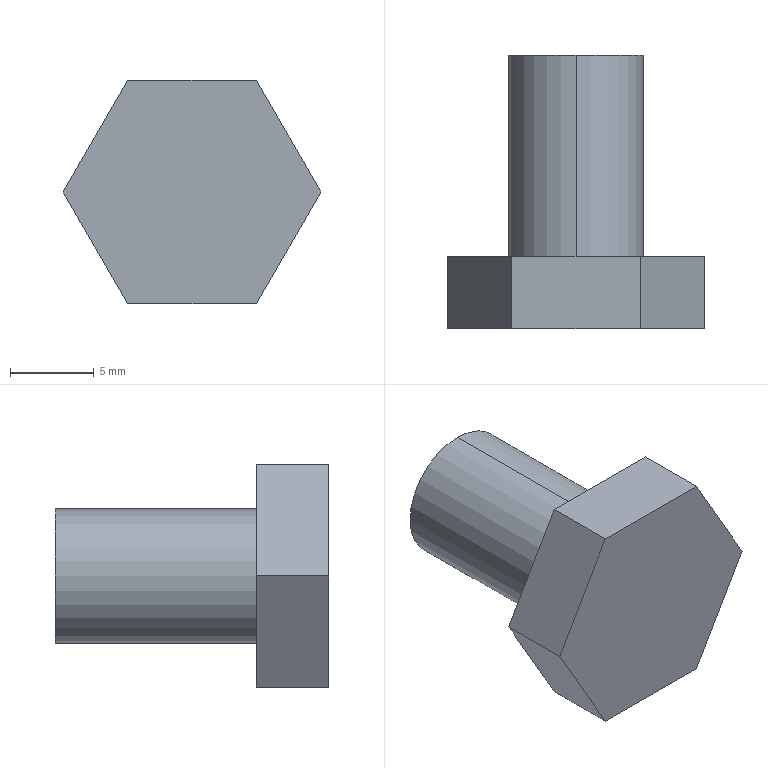Part | SolidWorks | features BaseBody 1 | 1 solid | 11 faces | box 15.358 x 16.3 x 13.3 mm | volume 1262 mm3 | plane 9 | cylinder 2 | commonest cylinder face diameters 8 x2
STEP:
#1=CARTESIAN_POINT('',(0.,16.3,-4.));
#2=VERTEX_POINT('',#1);
#3=CARTESIAN_POINT('',(0.,16.3,4.));
#4=VERTEX_POINT('',#3);
#5=CARTESIAN_POINT('',(0.,16.3,0.));
#6=DIRECTION('',(0.,-1.,0.));
#7=DIRECTION('',(0.,0.,-1.));
#8=AXIS2_PLACEMENT_3D('',#5,#6,#7);
#9=CIRCLE('',#8,4.);
#10=EDGE_CURVE('',#2,#4,#9,.T.);
#11=ORIENTED_EDGE('',*,*,#10,.T.);
#12=CARTESIAN_POINT('',(0.,4.3,4.));
#13=VERTEX_POINT('',#12);
#14=CARTESIAN_POINT('',(0.,16.3,4.));
#15=DIRECTION('',(0.,-1.,0.));
#16=VECTOR('',#15,1000.);
#17=LINE('',#14,#16);
#18=EDGE_CURVE('',#4,#13,#17,.T.);
#19=ORIENTED_EDGE('',*,*,#18,.T.);
#20=CARTESIAN_POINT('',(0.,4.3,-4.));
#21=VERTEX_POINT('',#20);
#22=CARTESIAN_POINT('',(0.,4.3,0.));
#23=DIRECTION('',(0.,-1.,0.));
#24=DIRECTION('',(0.,0.,-1.));
#25=AXIS2_PLACEMENT_3D('',#22,#23,#24);
#26=CIRCLE('',#25,4.);
#27=EDGE_CURVE('',#21,#13,#26,.T.);
#28=ORIENTED_EDGE('',*,*,#27,.F.);
#29=CARTESIAN_POINT('',(0.,16.3,-4.));
#30=DIRECTION('',(0.,-1.,0.));
#31=VECTOR('',#30,1000.);
#32=LINE('',#29,#31);
#33=EDGE_CURVE('',#2,#21,#32,.T.);
#34=ORIENTED_EDGE('',*,*,#33,.F.);
#35=EDGE_LOOP('',(#11,#19,#28,#34));
#36=FACE_OUTER_BOUND('',#35,.T.);
#37=CARTESIAN_POINT('',(0.,16.3,0.));
#38=DIRECTION('',(0.,-1.,0.));
#39=DIRECTION('',(0.,0.,-1.));
#40=AXIS2_PLACEMENT_3D('',#37,#38,#39);
#41=CYLINDRICAL_SURFACE('',#40,4.);
#42=ADVANCED_FACE('',(#36),#41,.T.);
#43=CARTESIAN_POINT('',(-3.839,0.,6.65));
#44=VERTEX_POINT('',#43);
#45=CARTESIAN_POINT('',(3.839,0.,6.65));
#46=VERTEX_POINT('',#45);
#47=CARTESIAN_POINT('',(0.,0.,6.65));
#48=DIRECTION('',(1.,0.,0.));
#49=VECTOR('',#48,1000.);
#50=LINE('',#47,#49);
#51=EDGE_CURVE('',#44,#46,#50,.T.);
#52=ORIENTED_EDGE('',*,*,#51,.F.);
#53=CARTESIAN_POINT('',(-7.679,0.,0.));
#54=VERTEX_POINT('',#53);
#55=CARTESIAN_POINT('',(-7.679,0.,0.));
#56=DIRECTION('',(0.5,0.,0.866));
#57=VECTOR('',#56,1000.);
#58=LINE('',#55,#57);
#59=EDGE_CURVE('',#54,#44,#58,.T.);
#60=ORIENTED_EDGE('',*,*,#59,.F.);
#61=CARTESIAN_POINT('',(-3.839,0.,-6.65));
#62=VERTEX_POINT('',#61);
#63=CARTESIAN_POINT('',(-3.839,0.,-6.65));
#64=DIRECTION('',(-0.5,0.,0.866));
#65=VECTOR('',#64,1000.);
#66=LINE('',#63,#65);
#67=EDGE_CURVE('',#62,#54,#66,.T.);
#68=ORIENTED_EDGE('',*,*,#67,.F.);
#69=CARTESIAN_POINT('',(3.839,0.,-6.65));
#70=VERTEX_POINT('',#69);
#71=CARTESIAN_POINT('',(0.,0.,-6.65));
#72=DIRECTION('',(-1.,0.,0.));
#73=VECTOR('',#72,1000.);
#74=LINE('',#71,#73);
#75=EDGE_CURVE('',#70,#62,#74,.T.);
#76=ORIENTED_EDGE('',*,*,#75,.F.);
#77=CARTESIAN_POINT('',(7.679,0.,0.));
#78=VERTEX_POINT('',#77);
#79=CARTESIAN_POINT('',(7.679,0.,0.));
#80=DIRECTION('',(-0.5,0.,-0.866));
#81=VECTOR('',#80,1000.);
#82=LINE('',#79,#81);
#83=EDGE_CURVE('',#78,#70,#82,.T.);
#84=ORIENTED_EDGE('',*,*,#83,.F.);
#85=CARTESIAN_POINT('',(3.839,0.,6.65));
#86=DIRECTION('',(0.5,0.,-0.866));
#87=VECTOR('',#86,1000.);
#88=LINE('',#85,#87);
#89=EDGE_CURVE('',#46,#78,#88,.T.);
#90=ORIENTED_EDGE('',*,*,#89,.F.);
#91=EDGE_LOOP('',(#52,#60,#68,#76,#84,#90));
#92=FACE_OUTER_BOUND('',#91,.T.);
#93=CARTESIAN_POINT('',(0.,0.,0.));
#94=DIRECTION('',(0.,1.,0.));
#95=DIRECTION('',(0.,0.,1.));
#96=AXIS2_PLACEMENT_3D('',#93,#94,#95);
#97=PLANE('',#96);
#98=ADVANCED_FACE('',(#92),#97,.F.);
#99=CARTESIAN_POINT('',(7.679,4.3,0.));
#100=VERTEX_POINT('',#99);
#101=CARTESIAN_POINT('',(7.679,4.3,0.));
#102=DIRECTION('',(0.,-1.,0.));
#103=VECTOR('',#102,1000.);
#104=LINE('',#101,#103);
#105=EDGE_CURVE('',#100,#78,#104,.T.);
#106=ORIENTED_EDGE('',*,*,#105,.F.);
#107=CARTESIAN_POINT('',(3.839,4.3,6.65));
#108=VERTEX_POINT('',#107);
#109=CARTESIAN_POINT('',(3.839,4.3,6.65));
#110=DIRECTION('',(0.5,0.,-0.866));
#111=VECTOR('',#110,1000.);
#112=LINE('',#109,#111);
#113=EDGE_CURVE('',#108,#100,#112,.T.);
#114=ORIENTED_EDGE('',*,*,#113,.F.);
#115=CARTESIAN_POINT('',(3.839,4.3,6.65));
#116=DIRECTION('',(0.,1.,0.));
#117=VECTOR('',#116,1000.);
#118=LINE('',#115,#117);
#119=EDGE_CURVE('',#46,#108,#118,.T.);
#120=ORIENTED_EDGE('',*,*,#119,.F.);
#121=ORIENTED_EDGE('',*,*,#89,.T.);
#122=EDGE_LOOP('',(#106,#114,#120,#121));
#123=FACE_OUTER_BOUND('',#122,.T.);
#124=CARTESIAN_POINT('',(3.839,4.3,6.65));
#125=DIRECTION('',(-0.866,0.,-0.5));
#126=DIRECTION('',(-0.5,0.,0.866));
#127=AXIS2_PLACEMENT_3D('',#124,#125,#126);
#128=PLANE('',#127);
#129=ADVANCED_FACE('',(#123),#128,.F.);
#130=ORIENTED_EDGE('',*,*,#119,.T.);
#131=CARTESIAN_POINT('',(-3.839,4.3,6.65));
#132=VERTEX_POINT('',#131);
#133=CARTESIAN_POINT('',(-3.839,4.3,6.65));
#134=DIRECTION('',(1.,0.,0.));
#135=VECTOR('',#134,1000.);
#136=LINE('',#133,#135);
#137=EDGE_CURVE('',#132,#108,#136,.T.);
#138=ORIENTED_EDGE('',*,*,#137,.F.);
#139=CARTESIAN_POINT('',(-3.839,4.3,6.65));
#140=DIRECTION('',(0.,1.,0.));
#141=VECTOR('',#140,1000.);
#142=LINE('',#139,#141);
#143=EDGE_CURVE('',#44,#132,#142,.T.);
#144=ORIENTED_EDGE('',*,*,#143,.F.);
#145=ORIENTED_EDGE('',*,*,#51,.T.);
#146=EDGE_LOOP('',(#130,#138,#144,#145));
#147=FACE_OUTER_BOUND('',#146,.T.);
#148=CARTESIAN_POINT('',(-3.839,4.3,6.65));
#149=DIRECTION('',(0.,0.,-1.));
#150=DIRECTION('',(-1.,0.,0.));
#151=AXIS2_PLACEMENT_3D('',#148,#149,#150);
#152=PLANE('',#151);
#153=ADVANCED_FACE('',(#147),#152,.F.);
#154=ORIENTED_EDGE('',*,*,#143,.T.);
#155=CARTESIAN_POINT('',(-7.679,4.3,0.));
#156=VERTEX_POINT('',#155);
#157=CARTESIAN_POINT('',(-7.679,4.3,0.));
#158=DIRECTION('',(0.5,0.,0.866));
#159=VECTOR('',#158,1000.);
#160=LINE('',#157,#159);
#161=EDGE_CURVE('',#156,#132,#160,.T.);
#162=ORIENTED_EDGE('',*,*,#161,.F.);
#163=CARTESIAN_POINT('',(-7.679,4.3,0.));
#164=DIRECTION('',(0.,1.,0.));
#165=VECTOR('',#164,1000.);
#166=LINE('',#163,#165);
#167=EDGE_CURVE('',#54,#156,#166,.T.);
#168=ORIENTED_EDGE('',*,*,#167,.F.);
#169=ORIENTED_EDGE('',*,*,#59,.T.);
#170=EDGE_LOOP('',(#154,#162,#168,#169));
#171=FACE_OUTER_BOUND('',#170,.T.);
#172=CARTESIAN_POINT('',(-7.679,4.3,0.));
#173=DIRECTION('',(0.866,0.,-0.5));
#174=DIRECTION('',(-0.5,0.,-0.866));
#175=AXIS2_PLACEMENT_3D('',#172,#173,#174);
#176=PLANE('',#175);
#177=ADVANCED_FACE('',(#171),#176,.F.);
#178=ORIENTED_EDGE('',*,*,#167,.T.);
#179=CARTESIAN_POINT('',(-3.839,4.3,-6.65));
#180=VERTEX_POINT('',#179);
#181=CARTESIAN_POINT('',(-3.839,4.3,-6.65));
#182=DIRECTION('',(-0.5,0.,0.866));
#183=VECTOR('',#182,1000.);
#184=LINE('',#181,#183);
#185=EDGE_CURVE('',#180,#156,#184,.T.);
#186=ORIENTED_EDGE('',*,*,#185,.F.);
#187=CARTESIAN_POINT('',(-3.839,4.3,-6.65));
#188=DIRECTION('',(0.,1.,0.));
#189=VECTOR('',#188,1000.);
#190=LINE('',#187,#189);
#191=EDGE_CURVE('',#62,#180,#190,.T.);
#192=ORIENTED_EDGE('',*,*,#191,.F.);
#193=ORIENTED_EDGE('',*,*,#67,.T.);
#194=EDGE_LOOP('',(#178,#186,#192,#193));
#195=FACE_OUTER_BOUND('',#194,.T.);
#196=CARTESIAN_POINT('',(-3.839,4.3,-6.65));
#197=DIRECTION('',(0.866,0.,0.5));
#198=DIRECTION('',(0.5,0.,-0.866));
#199=AXIS2_PLACEMENT_3D('',#196,#197,#198);
#200=PLANE('',#199);
#201=ADVANCED_FACE('',(#195),#200,.F.);
#202=ORIENTED_EDGE('',*,*,#191,.T.);
#203=CARTESIAN_POINT('',(3.839,4.3,-6.65));
#204=VERTEX_POINT('',#203);
#205=CARTESIAN_POINT('',(3.839,4.3,-6.65));
#206=DIRECTION('',(-1.,0.,0.));
#207=VECTOR('',#206,1000.);
#208=LINE('',#205,#207);
#209=EDGE_CURVE('',#204,#180,#208,.T.);
#210=ORIENTED_EDGE('',*,*,#209,.F.);
#211=CARTESIAN_POINT('',(3.839,4.3,-6.65));
#212=DIRECTION('',(0.,1.,0.));
#213=VECTOR('',#212,1000.);
#214=LINE('',#211,#213);
#215=EDGE_CURVE('',#70,#204,#214,.T.);
#216=ORIENTED_EDGE('',*,*,#215,.F.);
#217=ORIENTED_EDGE('',*,*,#75,.T.);
#218=EDGE_LOOP('',(#202,#210,#216,#217));
#219=FACE_OUTER_BOUND('',#218,.T.);
#220=CARTESIAN_POINT('',(3.839,4.3,-6.65));
#221=DIRECTION('',(0.,0.,1.));
#222=DIRECTION('',(1.,0.,0.));
#223=AXIS2_PLACEMENT_3D('',#220,#221,#222);
#224=PLANE('',#223);
#225=ADVANCED_FACE('',(#219),#224,.F.);
#226=ORIENTED_EDGE('',*,*,#215,.T.);
#227=CARTESIAN_POINT('',(7.679,4.3,0.));
#228=DIRECTION('',(-0.5,0.,-0.866));
#229=VECTOR('',#228,1000.);
#230=LINE('',#227,#229);
#231=EDGE_CURVE('',#100,#204,#230,.T.);
#232=ORIENTED_EDGE('',*,*,#231,.F.);
#233=ORIENTED_EDGE('',*,*,#105,.T.);
#234=ORIENTED_EDGE('',*,*,#83,.T.);
#235=EDGE_LOOP('',(#226,#232,#233,#234));
#236=FACE_OUTER_BOUND('',#235,.T.);
#237=CARTESIAN_POINT('',(7.679,4.3,0.));
#238=DIRECTION('',(-0.866,0.,0.5));
#239=DIRECTION('',(0.5,0.,0.866));
#240=AXIS2_PLACEMENT_3D('',#237,#238,#239);
#241=PLANE('',#240);
#242=ADVANCED_FACE('',(#236),#241,.F.);
#243=ORIENTED_EDGE('',*,*,#161,.T.);
#244=ORIENTED_EDGE('',*,*,#137,.T.);
#245=ORIENTED_EDGE('',*,*,#113,.T.);
#246=ORIENTED_EDGE('',*,*,#231,.T.);
#247=ORIENTED_EDGE('',*,*,#209,.T.);
#248=ORIENTED_EDGE('',*,*,#185,.T.);
#249=EDGE_LOOP('',(#243,#244,#245,#246,#247,#248));
#250=FACE_OUTER_BOUND('',#249,.T.);
#251=ORIENTED_EDGE('',*,*,#27,.T.);
#252=CARTESIAN_POINT('',(0.,4.3,0.));
#253=DIRECTION('',(0.,-1.,0.));
#254=DIRECTION('',(0.,0.,-1.));
#255=AXIS2_PLACEMENT_3D('',#252,#253,#254);
#256=CIRCLE('',#255,4.);
#257=EDGE_CURVE('',#13,#21,#256,.T.);
#258=ORIENTED_EDGE('',*,*,#257,.T.);
#259=EDGE_LOOP('',(#251,#258));
#260=FACE_BOUND('',#259,.T.);
#261=CARTESIAN_POINT('',(0.,4.3,0.));
#262=DIRECTION('',(0.,1.,0.));
#263=DIRECTION('',(0.,0.,1.));
#264=AXIS2_PLACEMENT_3D('',#261,#262,#263);
#265=PLANE('',#264);
#266=ADVANCED_FACE('',(#250,#260),#265,.T.);
#267=ORIENTED_EDGE('',*,*,#18,.F.);
#268=CARTESIAN_POINT('',(0.,16.3,0.));
#269=DIRECTION('',(0.,-1.,0.));
#270=DIRECTION('',(0.,0.,-1.));
#271=AXIS2_PLACEMENT_3D('',#268,#269,#270);
#272=CIRCLE('',#271,4.);
#273=EDGE_CURVE('',#4,#2,#272,.T.);
#274=ORIENTED_EDGE('',*,*,#273,.T.);
#275=ORIENTED_EDGE('',*,*,#33,.T.);
#276=ORIENTED_EDGE('',*,*,#257,.F.);
#277=EDGE_LOOP('',(#267,#274,#275,#276));
#278=FACE_OUTER_BOUND('',#277,.T.);
#279=CARTESIAN_POINT('',(0.,16.3,0.));
#280=DIRECTION('',(0.,-1.,0.));
#281=DIRECTION('',(0.,0.,-1.));
#282=AXIS2_PLACEMENT_3D('',#279,#280,#281);
#283=CYLINDRICAL_SURFACE('',#282,4.);
#284=ADVANCED_FACE('',(#278),#283,.T.);
#285=ORIENTED_EDGE('',*,*,#10,.F.);
#286=ORIENTED_EDGE('',*,*,#273,.F.);
#287=EDGE_LOOP('',(#285,#286));
#288=FACE_OUTER_BOUND('',#287,.T.);
#289=CARTESIAN_POINT('',(0.,16.3,0.));
#290=DIRECTION('',(0.,1.,0.));
#291=DIRECTION('',(0.,0.,1.));
#292=AXIS2_PLACEMENT_3D('',#289,#290,#291);
#293=PLANE('',#292);
#294=ADVANCED_FACE('',(#288),#293,.T.);
#295=CLOSED_SHELL('',(#42,#98,#129,#153,#177,#201,#225,#242,#266,#284,#294));
#296=MANIFOLD_SOLID_BREP('',#295);
#297=CARTESIAN_POINT('',(0.,0.,0.));
#298=DIRECTION('',(0.,0.,1.));
#299=DIRECTION('',(1.,0.,0.));
#300=AXIS2_PLACEMENT_3D('',#297,#298,#299);
#301=(LENGTH_UNIT()NAMED_UNIT(*)SI_UNIT(.MILLI.,.METRE.));
#302=UNCERTAINTY_MEASURE_WITH_UNIT(LENGTH_MEASURE(0.00001),#301,'','');
#303=(NAMED_UNIT(*)PLANE_ANGLE_UNIT()SI_UNIT($,.RADIAN.));
#304=(NAMED_UNIT(*)SI_UNIT($,.STERADIAN.)SOLID_ANGLE_UNIT());
#305=(GEOMETRIC_REPRESENTATION_CONTEXT(3)GLOBAL_UNCERTAINTY_ASSIGNED_CONTEXT((#302))GLOBAL_UNIT_ASSIGNED_CONTEXT((#301,#303,#304))REPRESENTATION_CONTEXT('',''));
#306=ADVANCED_BREP_SHAPE_REPRESENTATION('',(#296,#300),#305);